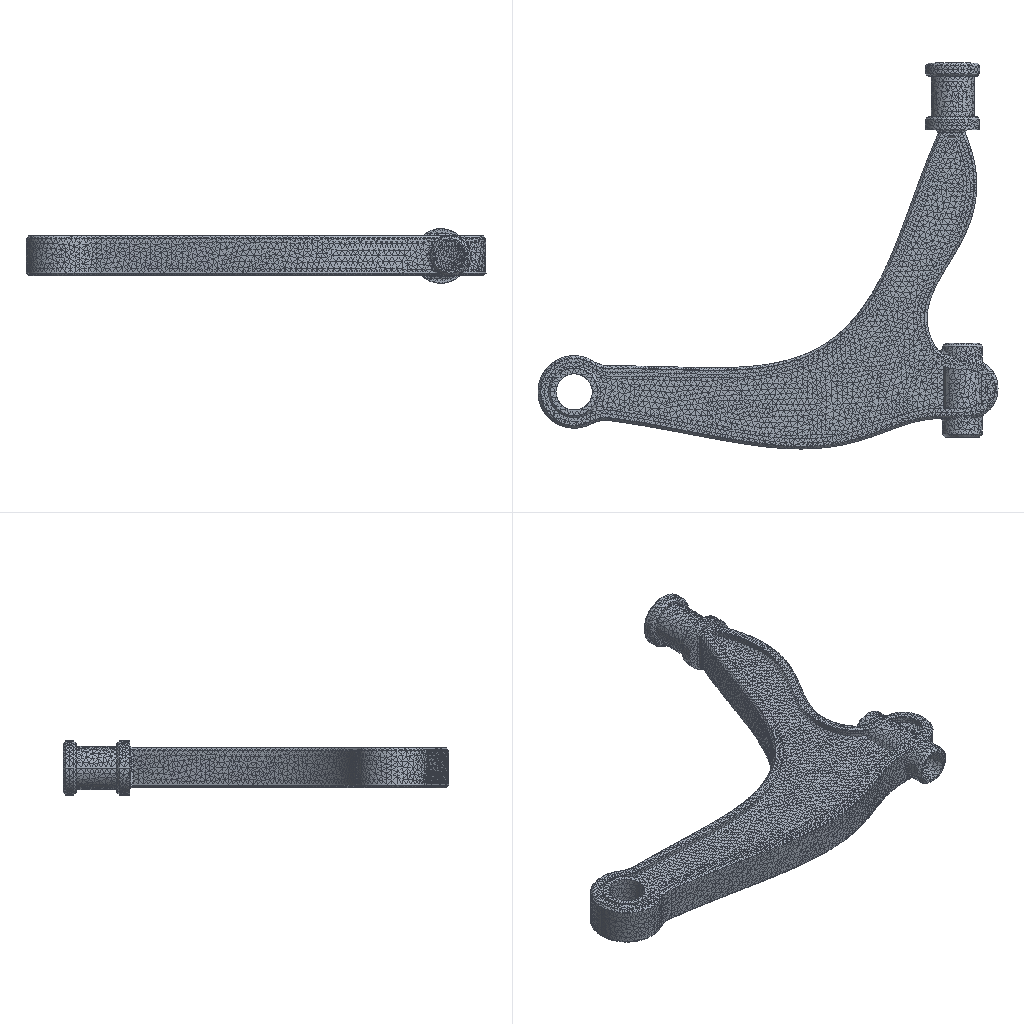Simulation study | ansys workbench
Ansys APDL input file, long lists of numbers shortened:
/batch
/config,noeldb,1     ! force off writing results to database
*get,_wallstrt,active,,time,wall
! ANSYS input file written by Workbench version 2023 R1
! File used for geometry attach:
/title,wbnew--__ (D5)
! ****** Begin Custom Load Command Snippet ******
/COM, ACT Extensions:
/COM,     LSDYNA, 2023.1
/COM,/COM,     ANSYSMotion, 2023.1
/COM,
! ****** End   Custom Load Command Snippet ******
*DIM,_wb_ProjectScratch_dir,string,248
_wb_ProjectScratch_dir(1) = ''
*DIM,_wb_SolverFiles_dir,string,248
_wb_SolverFiles_dir(1) = ''
*DIM,_wb_userfiles_dir,string,248
_wb_userfiles_dir(1) = ''
/com,--- Data in consistent NMM units. See Solving Units in the help system for more information.
/units,MPA
/nopr
/wb,file,start              !  signify a WB generated input file
/prep7
! Turn off shape checking because checks already performed inside WB mesher.
! See help system for more information.
SHPP,OFF,,NOWARN
/nolist
etcon,set             ! allow ANSYS to choose best KEYOP's for 180x elements, resets any applicable keyopt to MAPDL defaults
/com,*********** Nodes for the whole assembly ***********
nblock,3,,159214
(1i9,3e20.9e3)
        1    -1.427203437E+03     5.898657467E+00    -7.459739675E+01
! (144739 more lines like these left out)
-1
/wb,elem,start            !  set before creation of elements
/com,*********** Elements for Body 1 "xia bi.9" ***********
et,1,187
eblock,19,solid,,92956
(19i9)
        1        1        1        1        0        0        0        0       10        0        1    16771    17532    20834    20818   130193   134361   130201   130200
! (185911 more lines like these left out)
-1
/wb,elem,end               !  done creating elements
/com,*********** Send User Defined Coordinate System(s) ***********
csys,0
toffst,273.15,  ! Temperature offset from absolute zero
/com,*********** Set Reference Temperature ***********
tref,22.
/wb,mat,start              !  starting to send materials
/com,*********** Send Materials ***********
MP,DENS,1,7.85e-09,	! tonne mm^-3
MP,EX,1,210000,	! tonne s^-2 mm^-1
MP,NUXY,1,0.3,
/wb,mat,end                !  done sending materials
!************************* Model Summary ********************
!xia bi.9,	高强度冷轧板钢,	matid,	1
!************************* End Model Summary ********************
! get the diagonal of the bounding box. Needed later for other things
*get,_xmin,node,,mnloc,x
*get,_ymin,node,,mnloc,y
*get,_zmin,node,,mnloc,z
*get,_xmax,node,,mxloc,x
*get,_ymax,node,,mxloc,y
*get,_zmax,node,,mxloc,z
_ASMDIAG=(_xmax-_xmin)*(_xmax-_xmin)+(_ymax-_ymin)*(_ymax-_ymin)+(_zmax-_zmin)*(_zmax-_zmin)
_ASMDIAG=SQRT(_ASMDIAG)
/wb,contact,start          !  starting to send contact
/wb,contact,end            !  done creating contacts
/golist
/wb,load,start             !  starting to send loads
/gst,on,on
fini
*get,_numnode,node,0,count
*get,_numelem,elem,0,count
*get, _MAXELEMNUM, elem, 0, NUM, MAX
*get, _MAXNODENUM, node, 0, NUM, MAX
*get, _MAXELEMTYPE, etyp, 0, NUM, MAX
*get, _MAXREALCONST, rcon, 0, NUM, MAX
/go
/wb,load,end               !  done creating loads
/com,--- Number of total nodes = %_numnode%
/com,--- Number of contact elements = 0
/com,--- Number of spring elements = 0
/com,--- Number of bearing elements = 0
/com,--- Number of solid elements = 92956
/com,--- Number of condensed parts = 0
/com,--- Number of total elements = %_numelem%
*get,_wallbsol,active,,time,wall
/solu
antype,2                   ! modal analysis
_thickRatio=  1     ! Ratio of thick parts in the model
modopt,lanb,10
outres,erase
outres,all,none
outres,nsol,all
mxpand                    ! default expand in case of complex solution
dmpopt,esav,no
dmpopt,emat,no
dmpopt,full,no
! *********** WB SOLVE COMMAND ***********
! check interactive state
*get,ANSINTER_,active,,int
*if,ANSINTER_,ne,0,then
/eof
*endif
solve
/com *************** Write FE CONNECTORS *********
CEWRITE,file,ce,,INTE
*get,_nmodalsolproc,active,0,numcpu
fini
/nopr
*get,_numnode,node,0,count
*get,_numelem,elem,0,count
*get, _MAXELEMNUM, elem, 0, NUM, MAX
*get, _MAXNODENUM, node, 0, NUM, MAX,,,INTERNAL
*get, _MAXELEMTYPE, etyp, 0, NUM, MAX
*get, _MAXREALCONST, rcon, 0, NUM, MAX
*get,_NSOLTHREADS,active,0,ntfs
*get,_NSOLPROCESSES,active,0,npfs
/gopr
*get,_wallasol,active,,time,wall
/post1
/nopr
*dim,_direction,CHAR,6,1
_direction(1) = 'X'
_direction(2) = 'Y'
_direction(3) = 'Z'
_direction(4) = 'ROTX'
_direction(5) = 'ROTY'
_direction(6) = 'ROTZ'
*get,_lastLS,active,0,set,LSTP
*get,_beginset,active,0,set,nset,first,_lastLS
*get,_endset,active,0,set,nset,last,_lastLS
_nummodes = 0
*if,_endset,gt,0,then
_nummodes = _endset - _beginset + 1
*endif
*do,i_mode,1,_nummodes
   *do,j_component,1,6
			*get,PFACT_%i_mode%_%j_component%,MODE,%i_mode%,PFACT,,DIREC,_direction(%j_component%)
   *enddo
*enddo
*dim,_tmdirection,CHAR,6,1
_tmdirection(1) = 'X'
_tmdirection(2) = 'Y'
_tmdirection(3) = 'Z'
_tmdirection(4) = 'X'
_tmdirection(5) = 'Y'
_tmdirection(6) = 'Z'
*do,j_component,1,6
    *if,j_component,gt,3,then
        *get,TOTALMASS_%j_component%,ELEM,0,IOR,_tmdirection(%j_component%)
    *else
        *get,TOTALMASS_%j_component%,ELEM,0,MTOT,_tmdirection(%j_component%)
    *endif
*enddo
/gopr
xmlo,ENCODING,ISO-8859-1
xmlo,parm
/xml,parm,xml
fini
/gopr
*get,_walldone,active,,time,wall
_preptime=(_wallbsol-_wallstrt)*3600
_solvtime=(_wallasol-_wallbsol)*3600
_posttime=(_walldone-_wallasol)*3600
_totaltim=(_walldone-_wallstrt)*3600
*get,_dlbratio,active,0,solu,dlbr
*get,_combtime,active,0,solu,comb
*get,_ssmode,active,0,solu,ssmm
*get,_ndofs,active,0,solu,ndof
/fclean				!clean distributed files
/com,--- Total number of nodes = %_numnode%
/com,--- Total number of elements = %_numelem%
/com,--- Element load balance ratio = %_dlbratio%
/com,--- Time to combine distributed files = %_combtime%
/com,--- Sparse memory mode = %_ssmode%
/com,--- Number of DOF = %_ndofs%
/wb,file,end               ! done with WB generated input